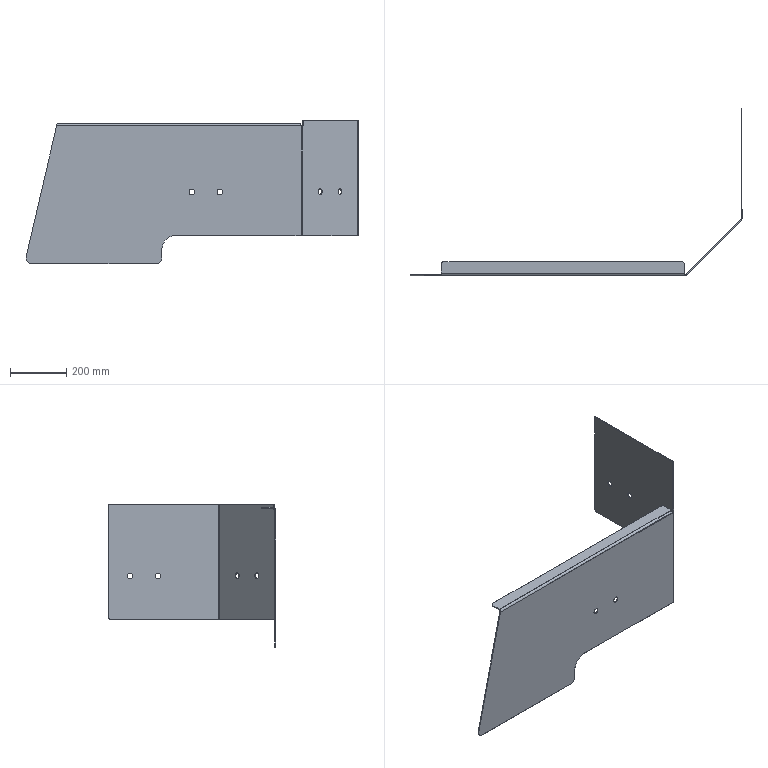Part | SolidWorks | features SM3dBend 3, FlatPattern 1, SMBaseFlange 1, SheetMetal 1 | 1 solid | 55 faces | box 1185 x 596.999 x 511 mm | volume 2337073 mm3 | cylinder 26 | plane 26 | spline 3 | commonest cylinder face diameters 20 x15 10 x5 16.4 x3 40 x2 100 x1